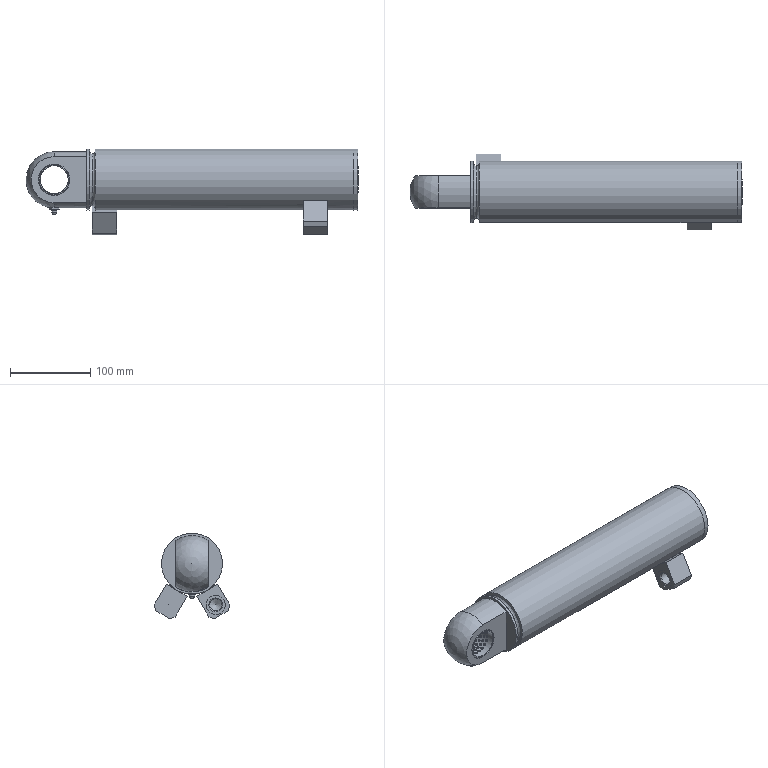Part | STEP file | HL7YG-5.59.024_抓具油缸(缸体)--000.002--20240512 | 11 solids | 238 faces | box 412.5 x 93.981 x 106.22 mm | volume 802630 mm3 | spline 100 | plane 64 | cylinder 45 | cone 23 | torus 3 | other 2 | sphere 1 | commonest cylinder face diameters 65 x7 32 x5 8 x4 36 x4 40 x4 76 x3